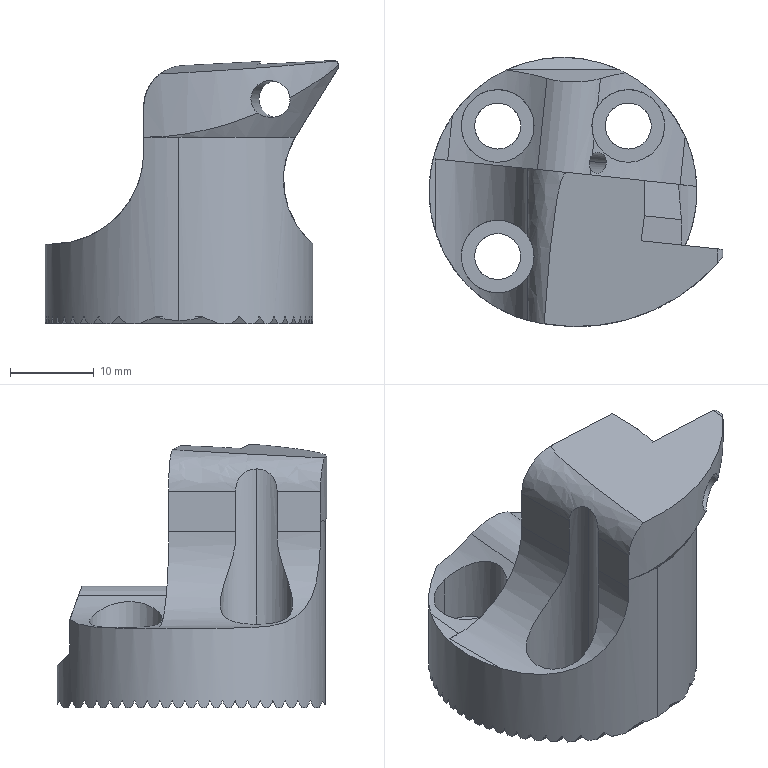NC program | Mastercam | posted with a generic post
Lines 1 to 726 of 7170:
%
:0001()
(MATERIAL - ALUMINUM MM - 2024)
(T4|12 FEMR |H4|XY STOCK TO LEAVE - 0.|Z STOCK TO LEAVE - .1)
(T1|8 FEM |H1)
(T2|2.5 DR |H2)
(T5|4 FEMR |H5|D5|WEAR COMP|TOOL DIA. - 4.|XY STOCK TO LEAVE - .05|Z STOCK TO LEAVE - .1)
(T6|3 FEMR |H6|D6|WEAR COMP|TOOL DIA. - 3.|XY STOCK TO LEAVE - .05|Z STOCK TO LEAVE - .1)
(T7|3 FEMF |H7|D7|WEAR COMP|TOOL DIA. - 3.|XY STOCK TO LEAVE - 0.|Z STOCK TO LEAVE - .01)
(T8|2 X 7 DCHC |H8|D8|WEAR COMP|TOOL DIA. - 6.)
(T9|12 FEMF |H9|D9|WEAR COMP|TOOL DIA. - 12.|XY STOCK TO LEAVE - 0.|Z STOCK TO LEAVE - .8)
(T10|30 BNOS |H10|D10|WEAR COMP|TOOL DIA. - 30.)
(T12|6 CHM |H12)
(T13|4.5 DR |H13)
(T11|5.5 FEM |H11)
(T14|2.4 THML |H14|D14|WEAR COMP|TOOL DIA. - 2.4)
(T15|2.5 BM |H15)
N100 G21
N102 G0 G17 G40 G80 G90 G94 G98
N104 G0 G28 G91 Z0.
N106 G0 G28 X0. Y0.
(12 FEMR |TOOL - 4|DIA. OFF. - 4|LEN. - 4|TOOL DIA. - 12.)
N108 T4 M6
N110 G0 G54 G90 X21.126 Y25.702 C6. B-90. S3500 M3
N112 G43 H4 Z51.893
N114 Z3.893
N116 G1 Z2.143 F600.
N118 X20.445 Y24.126 Z1.992 F2500.
N120 G3 X20.224 Y23.056 Z1.895 I2.479 J-1.07
N122 G1 Y23.028 Z1.893
N124 X20.231 Y22.429
N126 G3 X20.604 Y22.385 I.373 J1.549
N128 X20.718 Y22.389 J1.593
N130 X23.759 Y22.559 I-.265 J32.088
N132 X32.822 Y23.453 I-92.76 J985.834
N134 G1 X33.219 Y23.494
N136 X38.182 Y23.996
N138 G2 X38.795 Y24.028 I.613 J-5.909
N140 X41.037 Y23.589 J-5.941
N142 X44.111 Y21.167 I-2.73 J-6.627
N144 X45.663 Y17.751 I-7.846 J-5.626
N146 X46.13 Y14.462 I-17.344 J-4.138
N148 X46.244 Y9.771 I-96.071 J-4.691
N150 X46.243 Y9.367 I-96.185
N152 X46.249 Y6.557 I-902.501 J-3.15
N154 G1 Y6.157
N156 X46.247 Y-16.929
N158 G2 X45.424 Y-19.745 I-6.018 J.229
N160 X42.638 Y-22.432 I-6.221 J3.663
N162 X39.129 Y-23.539 I-4.677 J8.712
N164 X36.886 Y-23.675 I-2.243 J18.455
N166 X35.853 Y-23.646 J18.591
N168 X30.387 Y-23.202 I5.891 J106.242
N170 X28.391 Y-23.003 I95.895 J973.51
N172 G1 X27.993 Y-22.963
N174 X20.233 Y-22.178
N176 X20.225 Y-22.976
N178 Y-23.004 Z1.895
N180 G3 X20.446 Y-24.074 Z1.967 I2.7
N182 G1 X21.126 Y-25.651 Z2.081
N184 G3 X21.573 Y-26.459 Z2.143 I4.343 J1.874
N186 X25.469 Y-28.507 I3.896 J2.682
N188 X26.758 Y-28.328 J4.73
N190 G1 X42.937 Y-23.748 F9500.
N192 G3 X47.854 Y-17.248 I-1.841 J6.502
N194 G1 X47.867 Y16.229
N196 Y16.232
N198 G3 X39.016 Y25.645 I-9.431
N200 G1 X22.617 Y26.654
N202 G3 X22.526 Y26.657 I-.091 J-1.481
N204 X21.683 Y26.394 J-1.484
N206 X21.164 Y25.761 Z2.088 I.843 J-1.221 F2500.
N208 G1 X21.126 Y25.674 Z2.081
N210 X20.445 Y24.097 Z1.967
N212 G3 X20.224 Y23.027 Z1.895 I2.479 J-1.07
N214 G1 Y22.999 Z1.893
N216 X20.231 Y22.401
N218 Y22.383
N220 G3 X20.963 Y22.279 I.823 J3.176
N222 X21.844 Y22.262 I.881 J22.489
N224 X23.854 Y22.352 J22.506
N226 X32.043 Y23.124 I-29.673 J358.544
N228 G1 X32.439 Y23.164
N230 X36.767 Y23.597
N232 G2 X37.316 Y23.617 I.549 J-7.575
N234 X42.594 Y21.484 J-7.595
N236 X44.901 Y17.922 I-6.601 J-6.804
N238 X45.689 Y14.644 I-13.665 J-5.019
N240 X45.956 Y10.497 I-37.917 J-4.528
N242 X46.003 Y2.253 I-721.504 J-8.244
N244 X46. Y.007 I-721.551
N246 G1 Y-.392
N248 X45.989 Y-15.414
N250 G2 X43.557 Y-20.614 I-7.566 J.37
N252 X39.773 Y-22.709 I-6.283 J6.886
N254 X36.103 Y-23.233 I-3.838 J13.773
N256 X35.546 Y-23.237 I-.557 J39.206
N258 X31.968 Y-23.073 J39.21
N260 X21.574 Y-22.063 I62.472 J697.271
N262 G3 X20.536 Y-22.014 I-1.038 J-11.066
N264 X20.235 Y-22.019 J-11.115
N266 G1 X20.231 Y-22.418
N268 X20.227 Y-22.817
N270 Y-22.845 Z1.895
N272 G3 X20.447 Y-23.915 Z1.967 I2.699
N274 G1 X21.128 Y-25.492 Z2.081
N276 G3 X21.576 Y-26.299 Z2.143 I4.245 J1.832
N278 X25.373 Y-28.284 I3.797 J2.639 F9500.
N280 X26.533 Y-28.135 J4.624
N282 G1 X42.44 Y-24.009
N284 G3 X47.384 Y-17.801 I-1.658 J6.393
N286 G1 X48.247 Y13.016
N288 G3 X48.252 Y13.355 I-12.108 J.339
N290 X37.169 Y25.423 I-12.113
N292 G1 X22.705 Y26.657
N294 G3 X22.576 Y26.662 I-.129 J-1.514
N296 X21.662 Y26.357 J-1.519
N298 X21.181 Y25.745 Z2.09 I.914 J-1.214 F2500.
N300 G1 X21.126 Y25.619 Z2.081
N302 X20.446 Y24.043 Z1.967
N304 G3 X20.225 Y22.973 Z1.895 I2.479 J-1.07
N306 G1 Y22.945 Z1.893
N308 X20.231 Y22.346
N310 X20.232 Y22.323
N312 G3 X20.946 Y22.174 I.969 J2.856
N314 X22.527 Y22.099 I1.581 J16.604
N316 X23.658 Y22.137 J16.679
N318 X29.758 Y22.647 I-8.584 J139.485
N320 X31.339 Y22.803 I-97.596 J992.158
N322 G1 X31.735 Y22.843
N324 G2 X35.462 Y23.211 I61.376 J-602.807
N326 X36.208 Y23.243 I.746 J-8.651
N328 X39.94 Y22.4 J-8.683
N330 X43.58 Y19.078 I-4.043 J-8.085
N332 X45.112 Y15.242 I-10.404 J-6.378
N334 X45.622 Y11.232 I-24.215 J-5.117
N336 X45.745 Y5.578 I-129.778 J-5.654
N338 X45.743 Y4.973 I-129.901
N340 X45.748 Y2.967 I-962.168 J-2.989
N342 G1 Y2.567
N344 X45.74 Y-13.988
N346 G2 X44.157 Y-18.783 I-8.574 J.171
N348 X40.378 Y-21.782 I-7.314 J5.336
N350 X36.783 Y-22.724 I-4.966 J11.632
N352 X34.188 Y-22.859 I-2.595 J24.827
N354 X32.755 Y-22.818 J24.962
N356 X26.521 Y-22.306 I7.673 J131.735
N358 X24.525 Y-22.108 I95.907 J976.492
N360 G1 X24.126 Y-22.068
N362 G3 X21.308 Y-21.836 I-4.729 J-40.142
N364 X21.089 Y-21.833 I-.219 J-8.992
N366 X20.236 Y-21.873 J-8.995
N368 G1 X20.232 Y-22.272
N370 X20.228 Y-22.672
N372 Y-22.7 Z1.895
N374 G3 X20.449 Y-23.769 Z1.967 I2.7
N376 G1 X21.129 Y-25.346 Z2.081
N378 G3 X21.577 Y-26.153 Z2.143 I4.286 J1.85
N380 X25.415 Y-28.164 I3.838 J2.657 F9500.
N382 X26.953 Y-27.904 J4.668
N384 G1 X42.577 Y-22.455
N386 G3 X46.944 Y-17.338 I-2.196 J6.297
N388 X47.143 Y-15.101 I-12.443 J2.237
N390 G1 Y-14.985
N392 X46.859 Y15.892
N394 G3 X39.265 Y24.571 I-8.85 J-.081
N396 G1 X23.424 Y26.841
N398 G3 X23.117 Y26.863 I-.307 J-2.145
N400 X21.661 Y26.301 J-2.167
N402 X21.127 Y25.554 Z2.081 I1.456 J-1.605 F2500.
N404 G1 X20.447 Y23.978 Z1.967
N406 G3 X20.226 Y22.908 Z1.895 I2.479 J-1.07
N408 G1 Y22.88 Z1.893
N410 X20.232 Y22.281
N412 Y22.254
N414 G3 X20.931 Y22.069 I1.084 J2.678
N416 X22.918 Y21.926 I1.987 J13.766
N418 X23.512 Y21.939 J13.909
N420 X28.72 Y22.303 I-3.064 J81.411
N422 X33.895 Y22.808 I-66.02 J703.412
N424 G2 X35.175 Y22.88 I1.28 J-11.365
N426 X37.093 Y22.717 J-11.437
N428 X42.642 Y19.275 I-1.69 J-8.918
N430 X44.549 Y15.453 I-9.42 J-7.087
N432 X45.285 Y11.281 I-20.099 J-5.693
N434 X45.477 Y6.114 I-73.694 J-5.328
N436 X45.501 Y-.642 I-966.681 J-6.756
N438 X45.499 Y-1.921 I-966.705
N440 G1 X45.5 Y-2.321
N442 X45.497 Y-12.356
N444 G2 X45.498 Y-12.468 I-11.299 J-.112
N446 X45.066 Y-15.562 I-11.3
N448 X41.046 Y-20.701 I-8.707 J2.669
N450 X37.056 Y-22.188 I-6.075 J10.202
N452 X33.461 Y-22.497 I-3.595 J20.725
N454 X32.843 Y-22.488 J21.034
N456 X27.282 Y-22.119 I2.395 J78.13
N458 X23.709 Y-21.776 I53.927 J579.789
N460 G3 X21.383 Y-21.648 I-2.326 J-21.006
N462 X21.15 Y-21.649 J-21.134
N464 X20.238 Y-21.734 I.414 J-9.296
N466 G1 X20.234 Y-22.133
N468 X20.229 Y-22.532
N470 Y-22.561 Z1.895
N472 G3 X20.45 Y-23.63 Z1.967 I2.7
N474 G1 X21.131 Y-25.207 Z2.081
N476 G3 X21.634 Y-25.977 Z2.143 I2.479 J1.07
N478 X23.61 Y-26.837 I1.976 J1.84 F9500.
N480 X26.229 Y-24.791 J2.7
N482 G2 X28.325 Y-23.154 I2.096 J-.523
N484 X28.508 Y-23.161 J-2.16
N486 G3 X33.371 Y-23.422 I5.579 J58.622
N488 X33.668 Y-23.424 I.297 J19.418
N490 X37.918 Y-22.953 J19.42
N492 X42.626 Y-20.724 I-2.612 J11.602
N494 X46.372 Y-13.598 I-6.212 J7.813
N496 X46.437 Y-11.766 I-25.589 J1.832
N498 X46.429 Y-11.102 I-25.654
N500 G1 Y-8.707
N502 X46.41 Y5.72
N504 Y5.788
N506 G3 X46.214 Y11.312 I-78.078
N508 X45.43 Y15.749 I-21.74 J-1.555
N510 X43.095 Y20.192 I-11.923 J-3.43
N512 X35.874 Y23.792 I-7.671 J-6.343
N514 X35.24 Y23.805 I-.634 J-15.34
N516 X33.355 Y23.689 J-15.353
N518 X32.169 Y23.571 I96.557 J-974.034
N520 G1 X32.168
N522 X28.364 Y23.213
N524 G2 X26.254 Y24.946 I.007 J2.16
N526 G3 X23.607 Y27.114 I-2.647 J-.532
N528 X21.631 Y26.254 J-2.7
N530 X21.128 Y25.483 Z2.081 I1.976 J-1.84 F2500.
N532 G1 X20.447 Y23.907 Z1.967
N534 G3 X20.226 Y22.837 Z1.895 I2.479 J-1.07
N536 G1 Y22.809 Z1.893
N538 X20.233 Y22.21
N540 Y22.181
N542 G3 X20.916 Y21.966 I1.178 J2.544
N544 X23.185 Y21.752 I2.269 J11.95
N546 X23.396 Y21.754 J12.164
N548 X28.115 Y22.01 I-.654 J55.736
N550 X33.365 Y22.493 I-30.733 J362.463
N552 G2 X34.367 Y22.535 I1.002 J-11.971
N554 X36.489 Y22.346 J-12.013
N556 X42.409 Y18.557 I-1.822 J-9.365
N558 X44.227 Y14.845 I-9.988 J-7.194
N560 X44.995 Y10.693 I-20.279 J-5.9
N562 X45.219 Y5.495 I-67.686 J-5.514
N564 X45.252 Y-2.57 I-994.495 J-8.065
N566 X45.25 Y-4.551 I-994.528
N568 G1 Y-4.95
N570 X45.244 Y-11.424
N572 G2 X44.918 Y-14.332 I-13.208 J.008
N574 X40.512 Y-20.301 I-9.267 J2.229
N576 X36.625 Y-21.778 I-6.244 J10.58
N578 X32.733 Y-22.145 I-3.892 J20.447
N580 X32.403 Y-22.143 J20.814
N582 X27.199 Y-21.846 I1.182 J66.626
N584 X24.413 Y-21.592 I40.007 J453.687
N586 G3 X21.762 Y-21.45 I-2.786 J-27.176
N588 G1 X21.732
N590 G3 X20.239 Y-21.599 J-7.559
N592 G1 X20.235 Y-21.998
N594 X20.231 Y-22.397
N596 Y-22.425 Z1.895
N598 G3 X20.452 Y-23.495 Z1.967 I2.7
N600 G1 X21.132 Y-25.072 Z2.081
N602 G3 X21.579 Y-25.879 Z2.143 I4.334 J1.871
N604 X25.466 Y-27.921 I3.887 J2.678 F9500.
N606 X27.402 Y-27.507 J4.72
N608 G1 X42.652 Y-20.65
N610 G3 X46.629 Y-14.639 I-2.765 J6.15
N612 G1 X47.145 Y10.39
N614 G3 X47.148 Y10.676 I-13.882 J.286
N616 X35.652 Y24.354 I-13.885
N618 G1 X22.911 Y26.58
N620 G3 X22.648 Y26.603 I-.263 J-1.504
N622 X21.605 Y26.191 J-1.527
N624 X21.246 Y25.681 Z2.101 I1.043 J-1.115 F2500.
N626 G1 X21.129 Y25.408 Z2.081
N628 X20.448 Y23.832 Z1.967
N630 G3 X20.227 Y22.762 Z1.895 I2.479 J-1.07
N632 G1 Y22.734 Z1.893
N634 X20.234 Y22.135
N636 Y22.104
N638 G3 X20.902 Y21.862 I1.259 J2.437
N640 X23.298 Y21.578 I2.494 J10.77
N642 X23.876 Y21.574 I.578 J42.885
N644 X27.544 Y21.731 J42.889
N646 X32.326 Y22.144 I-20.553 J265.983
N648 G2 X33.566 Y22.2 I1.24 J-13.807
N650 X35.476 Y22.067 J-13.863
N652 X42.175 Y17.886 I-1.481 J-9.83
N654 X44.002 Y13.985 I-10.728 J-7.404
N656 X44.732 Y9.906 I-21.603 J-5.97
N658 X44.97 Y4.303 I-70.443 J-5.788
N660 X45.001 Y-3.307 I-925.209 J-7.61
N662 X44.999 Y-4.94 I-925.24
N664 G1 Y-5.34
N666 G2 X45. Y-6.617 I-611.888 J-1.277
N668 X44.988 Y-10.649 I-611.889
N670 X44.607 Y-13.784 I-13.796 J.083
N672 X39.789 Y-20.049 I-9.647 J2.434
N674 X35.72 Y-21.483 I-6.303 J11.392
N676 X31.944 Y-21.804 I-3.776 J22.021
N678 X31.585 Y-21.801 J22.342
N680 X26.402 Y-21.511 I1.25 J68.695
N682 G1 X26. Y-21.477
N684 G3 X22.422 Y-21.249 I-4.871 J-48.434
N686 X22.197 Y-21.246 I-.225 J-8.81
N688 X20.241 Y-21.466 J-8.813
N690 G1 X20.236 Y-21.865
N692 X20.232 Y-22.264
N694 Y-22.293 Z1.895
N696 G3 X20.453 Y-23.362 Z1.967 I2.7
N698 G1 X21.133 Y-24.939 Z2.081
N700 G3 X21.581 Y-25.747 Z2.143 I4.311 J1.86
N702 X25.444 Y-27.774 I3.863 J2.668 F9500.
N704 X27.489 Y-27.305 J4.695
N706 G1 X42.421 Y-20.079
N708 G3 X46.153 Y-14.885 I-2.921 J6.037
N710 X46.246 Y-13.524 I-11.661 J1.477
N712 G1 X46.499 Y11.891
N714 X46.471 Y12.827
N716 X46.369 Y13.758
N718 X46.192 Y14.678
N720 X45.943 Y15.581
N722 X45.623 Y16.462
N724 X45.234 Y17.314
N726 X44.778 Y18.132
N728 X44.259 Y18.912
N730 X43.679 Y19.647
N732 X43.042 Y20.334
N734 X42.353 Y20.968
N736 X41.615 Y21.546
N738 X40.834 Y22.063
N740 X40.014 Y22.515
N742 X39.161 Y22.902
N744 X38.279 Y23.219
N746 X37.375 Y23.463
N748 X23.66 Y26.612
N750 G3 X23.164 Y26.668 I-.496 J-2.16
N752 X21.66 Y26.079 J-2.216
N754 X21.129 Y25.33 Z2.081 I1.504 J-1.627 F2500.
N756 G1 X20.449 Y23.753 Z1.967
N758 G3 X20.228 Y22.684 Z1.895 I2.479 J-1.069
N760 G1 Y22.656 Z1.893
N762 X20.234 Y22.057
N764 X20.235 Y22.025
N766 G3 X20.888 Y21.76 I1.323 J2.324
N768 X23.212 Y21.409 I2.669 J9.82
N770 X24.574 Y21.383 I1.362 J36.185
N772 X27.375 Y21.492 J36.211
N774 X31.315 Y21.804 I-12.024 J176.847
N776 G2 X32.809 Y21.873 I1.494 J-16.046
N778 X34.495 Y21.785 J-16.115
N780 X41.945 Y17.246 I-1.13 J-10.237
N782 X43.782 Y13.152 I-11.394 J-7.573
N784 X44.515 Y8.674 I-23.669 J-6.17
N786 X44.725 Y2.723 I-88.134 J-6.098
N788 X44.749 Y-4.251 I-997.772 J-6.974
N790 G1 Y-5.309
N792 Y-5.708
N794 G2 X44.752 Y-6.738 I-180.422 J-1.03
N796 X44.716 Y-10.33 I-180.425
N798 X44.126 Y-13.865 I-13.238 J.395
N800 X39.483 Y-19.581 I-9.749 J3.176
N802 X35.467 Y-21.076 I-6.538 J11.418
N804 X31.362 Y-21.467 I-4.105 J21.366
N806 G1 X31.304
N808 G2 X26.502 Y-21.252 I.213 J58.586
N810 G1 X26.101 Y-21.222
N812 G3 X22.559 Y-21.045 I-3.943 J-43.363
N814 G1 X22.503
N816 G3 X20.668 Y-21.23 J-9.199
N818 G2 X20.242 Y-21.335 I-2.722 J10.097
N820 G1 X20.238 Y-21.734
N822 X20.234 Y-22.133
N824 Y-22.161 Z1.895
N826 G3 X20.454 Y-23.231 Z1.967 I2.7
N828 G1 X21.135 Y-24.808 Z2.081
N830 G3 X21.581 Y-25.616 Z2.143 I4.367 J1.885
N832 X25.502 Y-27.68 I3.921 J2.693 F9500.
N834 X27.779 Y-27.098 J4.757
N836 G1 X42.514 Y-19.061
N838 G3 X46.047 Y-13.416 I-3.253 J5.965
N840 G1 X46.941 Y5.535
N842 G3 X46.963 Y6.478 I-19.998 J.943
N844 X26.943 Y26.498 I-20.02
N846 G1 X22.023
N848 G3 X21.529 Y26.172 J-.539
N850 G1 X21.497 Y26.098
N852 X21.13 Y25.249 Z2.081 F2500.
N854 X20.45 Y23.673 Z1.967
N856 G3 X20.229 Y22.603 Z1.895 I2.479 J-1.07
N858 G1 Y22.575 Z1.893
N860 X20.235 Y21.976
N862 X20.236 Y21.943
N864 G3 X20.874 Y21.657 I1.392 J2.256
N866 X23.135 Y21.246 I2.821 J9.101
N868 X25.075 Y21.186 I1.94 J31.432
N870 X27.221 Y21.26 J31.492
N872 X30.774 Y21.506 I-8.983 J155.333
N874 G2 X32.103 Y21.556 I1.329 J-17.47
N876 X33.874 Y21.467 J-17.52
N878 X41.706 Y16.646 I-1.107 J-10.571
N880 X43.561 Y12.354 I-11.931 J-7.704
N882 X44.259 Y7.931 I-25.063 J-6.219
N884 X44.473 Y1.987 I-89.309 J-6.189
N886 X44.5 Y-5.225 I-953.14 J-7.212
N888 X44.499 Y-6.448 I-953.167
N890 X44.503 Y-7.132 I-64.488 J-.684
N892 X44.44 Y-9.966 I-64.492
N894 X43.784 Y-13.478 I-13.284 J.665
N896 X38.935 Y-19.274 I-10.016 J3.454
N898 X34.709 Y-20.781 I-6.643 J11.947
N900 X30.608 Y-21.142 I-4.101 J23.086
N902 X30.139 Y-21.138 J23.447
N904 X25.486 Y-20.921 I1.617 J84.754
N906 G3 X23.215 Y-20.839 I-2.271 J-31.287
N908 X22.434 Y-20.848 J-31.369
N910 X20.243 Y-21.205 I.195 J-8.107
N912 G1 X20.239 Y-21.604
N914 X20.235 Y-22.003
N916 Y-22.031 Z1.895
N918 G3 X20.456 Y-23.101 Z1.967 I2.7
N920 G1 X21.136 Y-24.677 Z2.081
N922 G3 X21.583 Y-25.485 Z2.143 I4.357 J1.88
N924 X25.493 Y-27.542 I3.91 J2.688 F9500.
N926 X27.891 Y-26.892 J4.745
N928 G1 X42.276 Y-18.47
N930 G3 X45.448 Y-14.182 I-3.425 J5.85
N932 X45.741 Y-11.669 I-10.612 J2.513
N934 X45.739 Y-11.422 I-10.905
N936 G1 X45.205 Y12.201
N938 G3 X38.317 Y22.094 I-10.903 J-.246
N940 G1 X25.736 Y27.077
N942 G3 X24.418 Y27.328 I-1.318 J-3.329
N944 X21.602 Y25.959 J-3.58
N946 X21.131 Y25.167 Z2.081 I2.816 J-2.211 F2500.
N948 G1 X20.451 Y23.59 Z1.967
N950 G3 X20.23 Y22.52 Z1.895 I2.479 J-1.07
N952 G1 Y22.492 Z1.893
N954 X20.236 Y21.893
N956 X20.237 Y21.859
N958 G3 X20.86 Y21.555 I1.469 J2.222
N960 X23.363 Y21.06 I3.128 J9.251
N962 X25.477 Y20.988 I2.114 J31.208
N964 X27.446 Y21.051 J31.28
N966 X29.799 Y21.192 I-7.885 J151.443
N968 G2 X31.365 Y21.248 I1.566 J-21.788
N970 X32.947 Y21.19 J-21.844
N972 X38.449 Y19.243 I-.854 J-11.161
N974 X42.138 Y14.892 I-6.667 J-9.391
N976 X43.571 Y10.529 I-14.835 J-7.292
N978 X44.093 Y5.862 I-34.127 J-6.179
N980 X44.24 Y-1.141 I-166.523 J-7.003
N982 G1 Y-1.575
N984 G2 X44.245 Y-3.582 I-933.219 J-3.552
N986 G1 X44.246 Y-3.982
N988 G2 X44.25 Y-5.151 I-186.966 J-1.169
N990 X44.219 Y-8.566 I-186.97
N992 X43.776 Y-12.022 I-15.739 J.259
N994 X38.12 Y-19.124 I-10.547 J2.596
N996 X33.987 Y-20.486 I-6.471 J12.69
N998 X29.95 Y-20.818 I-4.037 J24.35
N1000 X29.476 Y-20.814 J24.682
N1002 X25.308 Y-20.659 I2.24 J116.466
N1004 G3 X23.832 Y-20.618 I-1.476 J-26.664
N1006 X22.332 Y-20.66 J-26.705
N1008 X20.715 Y-20.922 I.546 J-8.489
N1010 G2 X20.245 Y-21.075 I-5.022 J14.679
N1012 G1 X20.241 Y-21.474
N1014 X20.236 Y-21.873
N1016 Y-21.901 Z1.895
N1018 G3 X20.457 Y-22.971 Z1.967 I2.7
N1020 G1 X21.138 Y-24.547 Z2.081
N1022 G3 X21.586 Y-25.354 Z2.143 I4.254 J1.835
N1024 X25.392 Y-27.345 I3.806 J2.642 F9500.
N1026 X27.742 Y-26.705 J4.633
N1028 G1 X41.669 Y-18.508
N1030 G3 X43.821 Y-16.472 I-3.357 J5.705
N1032 X45.518 Y-10.862 I-8.424 J5.61
N1034 X45.515 Y-10.615 I-10.121
N1036 G1 X44.983 Y11.197
N1038 G3 X44.112 Y15.064 I-10.119 J-.247
N1040 X34.614 Y23.343 I-13.648 J-6.071
N1042 G1 X23.969 Y26.421
N1044 G3 X23.31 Y26.514 I-.659 J-2.279
N1046 X21.653 Y25.839 J-2.372
N1048 X21.132 Y25.082 Z2.081 I1.657 J-1.697 F2500.
N1050 G1 X20.452 Y23.505 Z1.967
N1052 G3 X20.231 Y22.436 Z1.895 I2.479 J-1.069
N1054 G1 Y22.408 Z1.893
N1056 X20.237 Y21.809
N1058 Y21.773
N1060 G3 X20.846 Y21.452 I1.457 J2.025
N1062 X23.291 Y20.9 I3.25 J8.697
N1064 X25.824 Y20.786 I2.533 J28.152
N1066 X27.314 Y20.825 J28.266
N1068 X29.281 Y20.916 I-10.197 J242.484
N1070 G2 X30.602 Y20.955 I1.321 J-22.554
N1072 X32.66 Y20.861 J-22.593
N1074 X38.041 Y18.897 I-1.126 J-11.442
N1076 X41.733 Y14.634 I-6.746 J-9.57
N1078 X43.239 Y10.284 I-14.633 J-7.504
N1080 X43.816 Y5.585 I-32.528 J-6.373
N1082 X43.986 Y-1.25 I-137.655 J-6.835
N1084 X43.985 Y-1.479 I-137.825
N1086 X43.995 Y-3.924 I-297.953 J-2.445
N1088 X43.972 Y-7.649 I-297.963
N1090 X43.563 Y-11.239 I-17.793 J.21
N1092 X37.666 Y-18.791 I-10.853 J2.395
N1094 X33.581 Y-20.141 I-6.551 J12.973
N1096 X29.369 Y-20.499 I-4.212 J24.614
N1098 X29.092 Y-20.497 J24.972
N1100 X24.994 Y-20.401 I1.111 J135.173
N1102 G3 X24.252 Y-20.388 I-.742 J-21.923
N1104 X22.116 Y-20.493 J-21.936
N1106 X20.246 Y-20.945 I.679 J-6.897
N1108 G1 X20.242 Y-21.344
N1110 X20.238 Y-21.743
N1112 Y-21.772 Z1.895
N1114 G3 X20.459 Y-22.841 Z1.967 I2.7
N1116 G1 X21.139 Y-24.418 Z2.081
N1118 G3 X21.642 Y-25.188 Z2.143 I2.479 J1.07
N1120 X23.618 Y-26.048 I1.976 J1.84 F9500.
N1122 X26.315 Y-23.478 J2.7
N1124 G2 X28.479 Y-21.416 I2.164 J-.105
N1126 X28.666 Y-21.424 J-2.167
N1128 G3 X29.218 Y-21.429 I.552 J27.965
N1130 X33.277 Y-21.134 J27.97
N1132 X38.174 Y-19.574 I-2.255 J15.545
N1134 X43.868 Y-13.356 I-5.469 J10.726
N1136 X44.82 Y-9.132 I-13.342 J5.226
N1138 X44.929 Y-6.099 I-42.33 J3.033
N1140 X44.925 Y-5.499 I-42.439
N1142 X44.927 Y-4.252 I-325.294 J1.247
N1144 X44.825 Y3.879 I-325.296
N1146 X44.411 Y8.991 I-44.956 J-1.073
N1148 X43.114 Y13.872 I-20.099 J-2.726
N1150 X39.755 Y18.718 I-12.387 J-5.
N1152 X33.021 Y21.753 I-8.132 J-9.056
N1154 X30.703 Y21.889 I-2.318 J-19.694
N1156 X29.653 Y21.861 J-19.83
N1158 X28.577 Y21.813 I3.032 J-80.503
N1160 G2 X28.472 Y21.81 I-.105 J2.157
N1162 X26.312 Y23.951 J2.16
N1164 G3 X23.612 Y26.626 I-2.7 J-.025
N1166 X21.636 Y25.766 J-2.7
N1168 X21.133 Y24.996 Z2.081 I1.976 J-1.84 F2500.
N1170 G1 X20.453 Y23.419 Z1.967
N1172 G3 X20.232 Y22.35 Z1.895 I2.479 J-1.069
N1174 G1 Y22.321 Z1.893
N1176 X20.238 Y21.723
N1178 Y21.686
N1180 G3 X20.832 Y21.35 I1.488 J1.936
N1182 X23.224 Y20.743 I3.361 J8.231
N1184 X26.025 Y20.582 I2.801 J24.345
N1186 X26.832 Y20.596 J24.506
N1188 X29.209 Y20.663 I-3.949 J181.776
N1190 G2 X29.993 Y20.679 I.784 J-19.473
N1192 X32.695 Y20.491 J-19.489
N1194 X41.013 Y14.938 I-1.598 J-11.4
N1196 X42.788 Y10.549 I-13.263 J-7.92
N1198 X43.505 Y5.755 I-28.573 J-6.723
N1200 X43.721 Y-.566 I-99.664 J-6.566
N1202 X43.741 Y-3.528 I-218.951 J-2.962
N1204 X43.71 Y-7.191 I-218.971
N1206 X43.28 Y-10.768 I-17.976 J.351
N1208 X36.94 Y-18.603 I-11.097 J2.496
N1210 X32.397 Y-19.931 I-6.544 J13.951
N1212 X28.482 Y-20.192 I-3.915 J29.28
N1214 X28.072 Y-20.189 J29.541
N1216 X25.254 Y-20.158 I.99 J216.829
N1218 G3 X24.789 Y-20.153 I-.465 J-23.855
N1220 X22.338 Y-20.28 J-23.86
N1222 X20.247 Y-20.816 I.673 J-6.966
N1224 G1 X20.243 Y-21.215
N1226 X20.239 Y-21.614
N1228 Y-21.642 Z1.895
N1230 G3 X20.46 Y-22.712 Z1.967 I2.7
N1232 G1 X21.14 Y-24.289 Z2.081
N1234 G3 X21.586 Y-25.097 Z2.143 I4.425 J1.91
N1236 X25.565 Y-27.198 I3.979 J2.718 F9500.
N1238 X28.397 Y-26.279 J4.819
N1240 G1 X41.99 Y-16.411
N1242 G3 X44.562 Y-12.741 I-4.045 J5.572
N1244 G1 X46.534 Y-5.878
N1246 G3 X47.514 Y1.083 I-24.227 J6.961
N1248 X22.307 Y26.29 I-25.207
N1250 G1 X22.292
N1252 G3 X21.507 Y25.774 J-.855
N1254 G1 X21.5 Y25.757
N1256 X21.134 Y24.908 Z2.081 F2500.
N1258 X20.453 Y23.332 Z1.967
N1260 G3 X20.232 Y22.262 Z1.895 I2.479 J-1.07
N1262 G1 Y22.234 Z1.893
N1264 X20.239 Y21.635
N1266 Y21.598
N1268 G3 X20.818 Y21.248 I1.53 J1.877
N1270 X23.16 Y20.59 I3.461 J7.826
N1272 X26.275 Y20.378 I3.115 J22.822
N1274 X26.729 Y20.383 J23.034
N1276 G2 X28.596 Y20.401 I1.867 J-95.012
N1278 X30.123 Y20.389 J-95.03
N1280 X34.013 Y19.79 I-.297 J-14.847
N1282 X40.43 Y14.962 I-3.409 J-11.212
N1284 X42.301 Y10.846 I-12.621 J-8.22
N1286 X43.135 Y6.415 I-24.107 J-6.828
N1288 X43.446 Y.384 I-71.293 J-6.705
N1290 X43.483 Y-3.493 I-202.243 J-3.877
N1292 X43.465 Y-6.239 I-202.28
N1294 X43.081 Y-9.941 I-20.376 J.24
N1296 X40.227 Y-15.578 I-11.537 J2.3
N1298 X35.376 Y-18.755 I-8.992 J8.442
N1300 X30.782 Y-19.749 I-6.07 J16.92
N1302 X27.147 Y-19.902 I-3.635 J43.068
N1304 X26.726 Y-19.901 J43.221
N1306 G3 X26.144 Y-19.897 I-.582 J-44.215
N1308 X23.165 Y-19.997 J-44.219
N1310 X20.721 Y-20.482 I.584 J-9.344
N1312 X20.249 Y-20.686 I6.271 J-15.17
N1314 G1 X20.245 Y-21.085
N1316 X20.24 Y-21.484
N1318 Y-21.512 Z1.895
N1320 G3 X20.461 Y-22.582 Z1.967 I2.7
N1322 G1 X21.142 Y-24.159 Z2.081
N1324 G3 X21.586 Y-24.968 Z2.143 I4.465 J1.927
N1326 X25.607 Y-27.096 I4.021 J2.736 F9500.
N1328 X28.593 Y-26.071 J4.864
N1330 G1 X41.945 Y-15.689
N1332 G3 X44.402 Y-11.964 I-4.265 J5.486
N1334 G1 X46.521 Y-3.871
N1336 G3 X47.305 Y2.214 I-23.236 J6.085
N1338 X23.285 Y26.233 I-24.02
N1340 X21.657 Y25.575 J-2.341
N1342 X21.135 Y24.819 Z2.081 I1.628 J-1.683 F2500.
N1344 G1 X20.454 Y23.243 Z1.967
N1346 G3 X20.233 Y22.173 Z1.895 I2.479 J-1.07
N1348 G1 Y22.145 Z1.893
N1350 X20.24 Y21.546
N1352 Y21.508
N1354 G3 X20.984 Y21.058 I1.847 J2.215
N1356 X23.383 Y20.393 I3.6 J8.329
N1358 X26.612 Y20.171 I3.229 J23.415
N1360 X26.639 Y20.172 J23.637
N1362 X28.218 Y20.16 I2.057 J167.138
N1364 G1 X28.304
N1366 G2 X31.782 Y19.91 J-24.326
N1368 X37.431 Y17.5 I-1.844 J-12.149
N1370 X40.994 Y13.05 I-7.825 J-9.916
N1372 X42.469 Y8.578 I-16.152 J-7.81
N1374 X43.065 Y3.496 I-35.577 J-6.743
N1376 X43.223 Y-3.112 I-137.961 J-6.608
N1378 X43.188 Y-6.196 I-138.119
N1380 X42.68 Y-10.014 I-18.468 J.514
N1382 X36.217 Y-17.895 I-11.444 J2.794
N1384 X32.014 Y-19.21 I-6.748 J14.2
N1386 X27.715 Y-19.597 I-4.83 J29.528
N1388 G3 X23.924 Y-19.725 I1.552 J-102.721
N1390 X21.421 Y-20.102 I.734 J-13.356
N1392 X20.25 Y-20.556 I1.385 J-5.315
N1394 G1 X20.246 Y-20.955
N1396 X20.242 Y-21.354
N1398 Y-21.382 Z1.895
N1400 G3 X20.463 Y-22.452 Z1.967 I2.7
N1402 G1 X21.143 Y-24.028 Z2.081
N1404 G3 X21.589 Y-24.837 Z2.143 I4.403 J1.9
N1406 X25.546 Y-26.923 I3.957 J2.709 F9500.
N1408 X28.512 Y-25.896 J4.795
N1410 G1 X41.59 Y-15.602
N1412 G3 X43.843 Y-12.413 I-4.237 J5.383
N1414 G1 X45.385 Y-7.85
N1416 G3 X46.73 Y.33 I-24.194 J8.18
N1418 X38.599 Y19.017 I-25.539
N1420 X37.722 Y19.681 I-3.67 J-3.939
N1422 G1 X26.551 Y26.458
N1424 G3 X24.596 Y27.005 I-1.955 J-3.222
N1426 X21.602 Y25.525 J-3.769
N1428 X21.136 Y24.729 Z2.081 I2.994 J-2.289 F2500.
N1430 G1 X20.455 Y23.153 Z1.967
N1432 G3 X20.234 Y22.083 Z1.895 I2.479 J-1.07
N1434 G1 Y22.055 Z1.893
N1436 X20.241 Y21.456
N1438 Y21.417
N1440 G3 X20.792 Y21.042 I1.588 J1.742
N1442 X23.041 Y20.291 I3.635 J7.149
N1444 X26.195 Y19.974 I3.622 J20.152
N1446 X28.167 Y19.916 I5.11 J139.506
N1448 G2 X31.779 Y19.552 I-.484 J-22.945
N1450 X37.835 Y16.527 I-2.291 J-12.162
N1452 X40.995 Y12.015 I-9.156 J-9.776
N1454 X42.336 Y7.381 I-18.187 J-7.775
N1456 X42.858 Y1.966 I-43.179 J-6.89
N1458 X42.962 Y-2.881 I-113.194 J-4.847
N1460 X42.927 Y-5.667 I-113.298
N1462 X42.433 Y-9.448 I-19.042 J.566
N1464 X35.889 Y-17.537 I-11.651 J2.735
N1466 X31.471 Y-18.917 I-6.987 J14.604
N1468 X27.262 Y-19.322 I-5.27 J32.724
N1470 X26.051 Y-19.374 I-14.199 J312.729
N1472 G3 X22.683 Y-19.655 I.738 J-29.208
N1474 X20.658 Y-20.219 I1.164 J-8.098
N1476 G2 X20.251 Y-20.425 I-16.589 J32.149
N1478 G1 X20.247 Y-20.824
N1480 X20.243 Y-21.223
N1482 Y-21.251 Z1.895
N1484 G3 X20.464 Y-22.321 Z1.967 I2.7
N1486 G1 X21.144 Y-23.898 Z2.081
N1488 G3 X21.59 Y-24.706 Z2.143 I4.412 J1.904
N1490 X25.556 Y-26.799 I3.966 J2.712 F9500.
N1492 X28.616 Y-25.699 J4.805
N1494 G1 X41.494 Y-15.063
N1496 G3 X43.912 Y-10.781 I-4.371 J5.293
N1498 G1 X45.205 Y-2.097
N1500 G3 X45.464 Y1.407 I-23.551 J3.504
N1502 X30.957 Y23.325 I-23.81
N1504 G1 X24.39 Y26.112
N1506 G3 X23.445 Y26.304 I-.945 J-2.225
N1508 X21.591 Y25.438 J-2.417
N1510 X21.226 Y24.845 Z2.096 I1.854 J-1.551 F2500.
N1512 G1 X21.137 Y24.638 Z2.081
N1514 X20.456 Y23.061 Z1.967